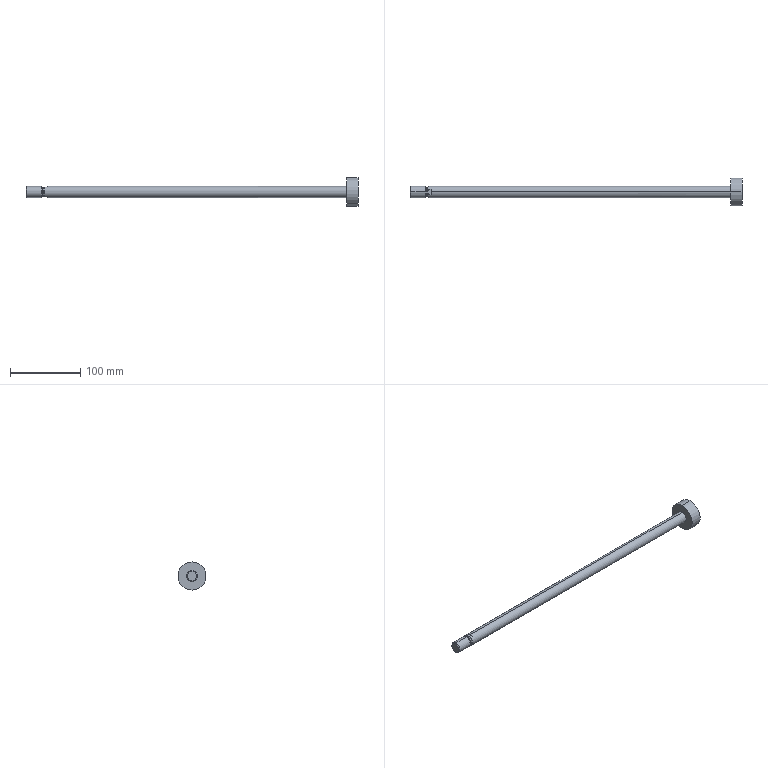Part | STEP file | 1 solid | 23 faces | box 471 x 40 x 40 mm | volume 111313 mm3 | plane 9 | cylinder 8 | cone 4 | torus 2 | commonest cylinder face diameters 16 x4 13.546 x2 40 x2